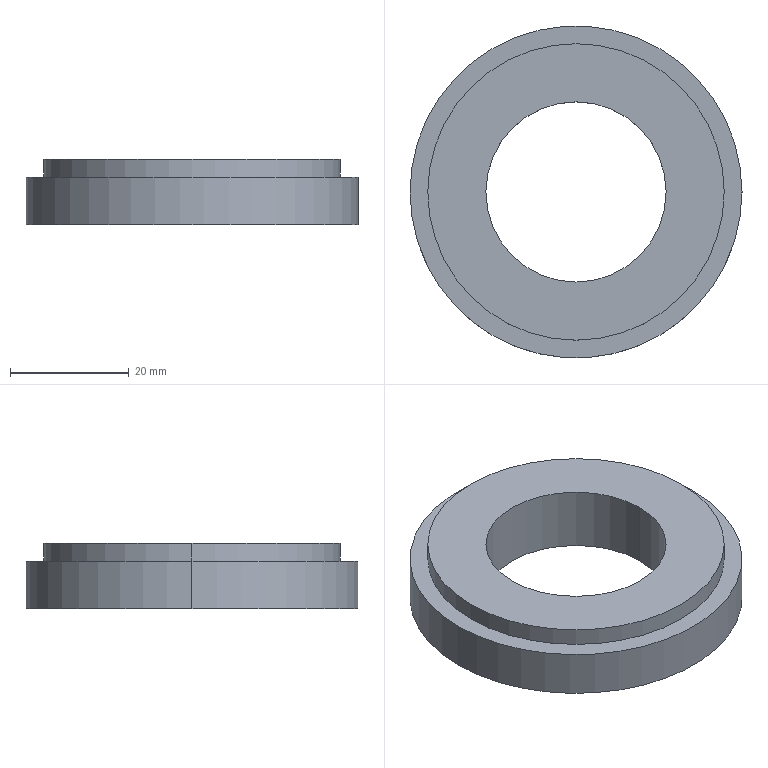Part | SolidWorks | features ICE 2, Extrusion 1 | 1 solid | 9 faces | box 56 x 56 x 11 mm | volume 17612 mm3 | cylinder 6 | plane 3 | commonest cylinder face diameters 30.397 x2 50 x2 56 x2
STEP:
#1=CARTESIAN_POINT('',(15.199,0.,11.));
#2=VERTEX_POINT('',#1);
#3=CARTESIAN_POINT('',(-15.199,0.,11.));
#4=VERTEX_POINT('',#3);
#5=CARTESIAN_POINT('',(0.,0.,11.));
#6=DIRECTION('',(0.,0.,-1.));
#7=DIRECTION('',(-1.,0.,0.));
#8=AXIS2_PLACEMENT_3D('',#5,#6,#7);
#9=CIRCLE('',#8,15.199);
#10=EDGE_CURVE('',#2,#4,#9,.T.);
#11=ORIENTED_EDGE('',*,*,#10,.F.);
#12=CARTESIAN_POINT('',(15.199,0.,0.));
#13=VERTEX_POINT('',#12);
#14=CARTESIAN_POINT('',(15.199,0.,11.));
#15=DIRECTION('',(0.,0.,-1.));
#16=VECTOR('',#15,1000.);
#17=LINE('',#14,#16);
#18=EDGE_CURVE('',#2,#13,#17,.T.);
#19=ORIENTED_EDGE('',*,*,#18,.T.);
#20=CARTESIAN_POINT('',(-15.199,0.,0.));
#21=VERTEX_POINT('',#20);
#22=CARTESIAN_POINT('',(0.,0.,0.));
#23=DIRECTION('',(0.,0.,-1.));
#24=DIRECTION('',(-1.,0.,0.));
#25=AXIS2_PLACEMENT_3D('',#22,#23,#24);
#26=CIRCLE('',#25,15.199);
#27=EDGE_CURVE('',#13,#21,#26,.T.);
#28=ORIENTED_EDGE('',*,*,#27,.T.);
#29=CARTESIAN_POINT('',(-15.199,0.,11.));
#30=DIRECTION('',(0.,0.,-1.));
#31=VECTOR('',#30,1000.);
#32=LINE('',#29,#31);
#33=EDGE_CURVE('',#4,#21,#32,.T.);
#34=ORIENTED_EDGE('',*,*,#33,.F.);
#35=EDGE_LOOP('',(#11,#19,#28,#34));
#36=FACE_OUTER_BOUND('',#35,.T.);
#37=CARTESIAN_POINT('',(0.,0.,11.));
#38=DIRECTION('',(0.,0.,-1.));
#39=DIRECTION('',(-1.,0.,0.));
#40=AXIS2_PLACEMENT_3D('',#37,#38,#39);
#41=CYLINDRICAL_SURFACE('',#40,15.199);
#42=ADVANCED_FACE('',(#36),#41,.F.);
#43=CARTESIAN_POINT('',(25.,0.,11.));
#44=VERTEX_POINT('',#43);
#45=CARTESIAN_POINT('',(-25.,0.,11.));
#46=VERTEX_POINT('',#45);
#47=CARTESIAN_POINT('',(0.,0.,11.));
#48=DIRECTION('',(0.,0.,1.));
#49=DIRECTION('',(1.,0.,0.));
#50=AXIS2_PLACEMENT_3D('',#47,#48,#49);
#51=CIRCLE('',#50,25.);
#52=EDGE_CURVE('',#44,#46,#51,.T.);
#53=ORIENTED_EDGE('',*,*,#52,.F.);
#54=CARTESIAN_POINT('',(25.,0.,8.));
#55=VERTEX_POINT('',#54);
#56=CARTESIAN_POINT('',(25.,0.,11.));
#57=DIRECTION('',(0.,0.,-1.));
#58=VECTOR('',#57,1000.);
#59=LINE('',#56,#58);
#60=EDGE_CURVE('',#44,#55,#59,.T.);
#61=ORIENTED_EDGE('',*,*,#60,.T.);
#62=CARTESIAN_POINT('',(-25.,0.,8.));
#63=VERTEX_POINT('',#62);
#64=CARTESIAN_POINT('',(0.,0.,8.));
#65=DIRECTION('',(0.,0.,1.));
#66=DIRECTION('',(1.,0.,0.));
#67=AXIS2_PLACEMENT_3D('',#64,#65,#66);
#68=CIRCLE('',#67,25.);
#69=EDGE_CURVE('',#55,#63,#68,.T.);
#70=ORIENTED_EDGE('',*,*,#69,.T.);
#71=CARTESIAN_POINT('',(-25.,0.,11.));
#72=DIRECTION('',(0.,0.,-1.));
#73=VECTOR('',#72,1000.);
#74=LINE('',#71,#73);
#75=EDGE_CURVE('',#46,#63,#74,.T.);
#76=ORIENTED_EDGE('',*,*,#75,.F.);
#77=EDGE_LOOP('',(#53,#61,#70,#76));
#78=FACE_OUTER_BOUND('',#77,.T.);
#79=CARTESIAN_POINT('',(0.,0.,11.));
#80=DIRECTION('',(0.,0.,-1.));
#81=DIRECTION('',(-1.,0.,0.));
#82=AXIS2_PLACEMENT_3D('',#79,#80,#81);
#83=CYLINDRICAL_SURFACE('',#82,25.);
#84=ADVANCED_FACE('',(#78),#83,.T.);
#85=CARTESIAN_POINT('',(28.,0.,8.));
#86=VERTEX_POINT('',#85);
#87=CARTESIAN_POINT('',(-28.,0.,8.));
#88=VERTEX_POINT('',#87);
#89=CARTESIAN_POINT('',(0.,0.,8.));
#90=DIRECTION('',(0.,0.,1.));
#91=DIRECTION('',(1.,0.,0.));
#92=AXIS2_PLACEMENT_3D('',#89,#90,#91);
#93=CIRCLE('',#92,28.);
#94=EDGE_CURVE('',#86,#88,#93,.T.);
#95=ORIENTED_EDGE('',*,*,#94,.F.);
#96=CARTESIAN_POINT('',(28.,0.,0.));
#97=VERTEX_POINT('',#96);
#98=CARTESIAN_POINT('',(28.,0.,8.));
#99=DIRECTION('',(0.,0.,-1.));
#100=VECTOR('',#99,1000.);
#101=LINE('',#98,#100);
#102=EDGE_CURVE('',#86,#97,#101,.T.);
#103=ORIENTED_EDGE('',*,*,#102,.T.);
#104=CARTESIAN_POINT('',(-28.,0.,0.));
#105=VERTEX_POINT('',#104);
#106=CARTESIAN_POINT('',(0.,0.,0.));
#107=DIRECTION('',(0.,0.,1.));
#108=DIRECTION('',(1.,0.,0.));
#109=AXIS2_PLACEMENT_3D('',#106,#107,#108);
#110=CIRCLE('',#109,28.);
#111=EDGE_CURVE('',#97,#105,#110,.T.);
#112=ORIENTED_EDGE('',*,*,#111,.T.);
#113=CARTESIAN_POINT('',(-28.,0.,8.));
#114=DIRECTION('',(0.,0.,-1.));
#115=VECTOR('',#114,1000.);
#116=LINE('',#113,#115);
#117=EDGE_CURVE('',#88,#105,#116,.T.);
#118=ORIENTED_EDGE('',*,*,#117,.F.);
#119=EDGE_LOOP('',(#95,#103,#112,#118));
#120=FACE_OUTER_BOUND('',#119,.T.);
#121=CARTESIAN_POINT('',(0.,0.,8.));
#122=DIRECTION('',(0.,0.,-1.));
#123=DIRECTION('',(-1.,0.,0.));
#124=AXIS2_PLACEMENT_3D('',#121,#122,#123);
#125=CYLINDRICAL_SURFACE('',#124,28.);
#126=ADVANCED_FACE('',(#120),#125,.T.);
#127=CARTESIAN_POINT('',(0.,0.,8.));
#128=DIRECTION('',(0.,0.,1.));
#129=DIRECTION('',(1.,0.,0.));
#130=AXIS2_PLACEMENT_3D('',#127,#128,#129);
#131=CIRCLE('',#130,28.);
#132=EDGE_CURVE('',#88,#86,#131,.T.);
#133=ORIENTED_EDGE('',*,*,#132,.T.);
#134=ORIENTED_EDGE('',*,*,#94,.T.);
#135=EDGE_LOOP('',(#133,#134));
#136=FACE_OUTER_BOUND('',#135,.T.);
#137=CARTESIAN_POINT('',(0.,0.,8.));
#138=DIRECTION('',(0.,0.,1.));
#139=DIRECTION('',(1.,0.,0.));
#140=AXIS2_PLACEMENT_3D('',#137,#138,#139);
#141=CIRCLE('',#140,25.);
#142=EDGE_CURVE('',#63,#55,#141,.T.);
#143=ORIENTED_EDGE('',*,*,#142,.F.);
#144=ORIENTED_EDGE('',*,*,#69,.F.);
#145=EDGE_LOOP('',(#143,#144));
#146=FACE_BOUND('',#145,.T.);
#147=CARTESIAN_POINT('',(0.,0.,8.));
#148=DIRECTION('',(0.,0.,1.));
#149=DIRECTION('',(1.,0.,0.));
#150=AXIS2_PLACEMENT_3D('',#147,#148,#149);
#151=PLANE('',#150);
#152=ADVANCED_FACE('',(#136,#146),#151,.T.);
#153=ORIENTED_EDGE('',*,*,#102,.F.);
#154=ORIENTED_EDGE('',*,*,#132,.F.);
#155=ORIENTED_EDGE('',*,*,#117,.T.);
#156=CARTESIAN_POINT('',(0.,0.,0.));
#157=DIRECTION('',(0.,0.,1.));
#158=DIRECTION('',(1.,0.,0.));
#159=AXIS2_PLACEMENT_3D('',#156,#157,#158);
#160=CIRCLE('',#159,28.);
#161=EDGE_CURVE('',#105,#97,#160,.T.);
#162=ORIENTED_EDGE('',*,*,#161,.T.);
#163=EDGE_LOOP('',(#153,#154,#155,#162));
#164=FACE_OUTER_BOUND('',#163,.T.);
#165=CARTESIAN_POINT('',(0.,0.,8.));
#166=DIRECTION('',(0.,0.,-1.));
#167=DIRECTION('',(-1.,0.,0.));
#168=AXIS2_PLACEMENT_3D('',#165,#166,#167);
#169=CYLINDRICAL_SURFACE('',#168,28.);
#170=ADVANCED_FACE('',(#164),#169,.T.);
#171=CARTESIAN_POINT('',(0.,0.,0.));
#172=DIRECTION('',(0.,0.,-1.));
#173=DIRECTION('',(-1.,0.,0.));
#174=AXIS2_PLACEMENT_3D('',#171,#172,#173);
#175=CIRCLE('',#174,15.199);
#176=EDGE_CURVE('',#21,#13,#175,.T.);
#177=ORIENTED_EDGE('',*,*,#176,.F.);
#178=ORIENTED_EDGE('',*,*,#27,.F.);
#179=EDGE_LOOP('',(#177,#178));
#180=FACE_BOUND('',#179,.T.);
#181=ORIENTED_EDGE('',*,*,#161,.F.);
#182=ORIENTED_EDGE('',*,*,#111,.F.);
#183=EDGE_LOOP('',(#181,#182));
#184=FACE_OUTER_BOUND('',#183,.T.);
#185=CARTESIAN_POINT('',(0.,0.,0.));
#186=DIRECTION('',(0.,0.,1.));
#187=DIRECTION('',(1.,0.,0.));
#188=AXIS2_PLACEMENT_3D('',#185,#186,#187);
#189=PLANE('',#188);
#190=ADVANCED_FACE('',(#180,#184),#189,.F.);
#191=ORIENTED_EDGE('',*,*,#60,.F.);
#192=CARTESIAN_POINT('',(0.,0.,11.));
#193=DIRECTION('',(0.,0.,1.));
#194=DIRECTION('',(1.,0.,0.));
#195=AXIS2_PLACEMENT_3D('',#192,#193,#194);
#196=CIRCLE('',#195,25.);
#197=EDGE_CURVE('',#46,#44,#196,.T.);
#198=ORIENTED_EDGE('',*,*,#197,.F.);
#199=ORIENTED_EDGE('',*,*,#75,.T.);
#200=ORIENTED_EDGE('',*,*,#142,.T.);
#201=EDGE_LOOP('',(#191,#198,#199,#200));
#202=FACE_OUTER_BOUND('',#201,.T.);
#203=CARTESIAN_POINT('',(0.,0.,11.));
#204=DIRECTION('',(0.,0.,-1.));
#205=DIRECTION('',(-1.,0.,0.));
#206=AXIS2_PLACEMENT_3D('',#203,#204,#205);
#207=CYLINDRICAL_SURFACE('',#206,25.);
#208=ADVANCED_FACE('',(#202),#207,.T.);
#209=CARTESIAN_POINT('',(0.,0.,11.));
#210=DIRECTION('',(0.,0.,-1.));
#211=DIRECTION('',(-1.,0.,0.));
#212=AXIS2_PLACEMENT_3D('',#209,#210,#211);
#213=CIRCLE('',#212,15.199);
#214=EDGE_CURVE('',#4,#2,#213,.T.);
#215=ORIENTED_EDGE('',*,*,#214,.T.);
#216=ORIENTED_EDGE('',*,*,#10,.T.);
#217=EDGE_LOOP('',(#215,#216));
#218=FACE_BOUND('',#217,.T.);
#219=ORIENTED_EDGE('',*,*,#197,.T.);
#220=ORIENTED_EDGE('',*,*,#52,.T.);
#221=EDGE_LOOP('',(#219,#220));
#222=FACE_OUTER_BOUND('',#221,.T.);
#223=CARTESIAN_POINT('',(0.,0.,11.));
#224=DIRECTION('',(0.,0.,1.));
#225=DIRECTION('',(1.,0.,0.));
#226=AXIS2_PLACEMENT_3D('',#223,#224,#225);
#227=PLANE('',#226);
#228=ADVANCED_FACE('',(#218,#222),#227,.T.);
#229=ORIENTED_EDGE('',*,*,#18,.F.);
#230=ORIENTED_EDGE('',*,*,#214,.F.);
#231=ORIENTED_EDGE('',*,*,#33,.T.);
#232=ORIENTED_EDGE('',*,*,#176,.T.);
#233=EDGE_LOOP('',(#229,#230,#231,#232));
#234=FACE_OUTER_BOUND('',#233,.T.);
#235=CARTESIAN_POINT('',(0.,0.,11.));
#236=DIRECTION('',(0.,0.,-1.));
#237=DIRECTION('',(-1.,0.,0.));
#238=AXIS2_PLACEMENT_3D('',#235,#236,#237);
#239=CYLINDRICAL_SURFACE('',#238,15.199);
#240=ADVANCED_FACE('',(#234),#239,.F.);
#241=CLOSED_SHELL('',(#42,#84,#126,#152,#170,#190,#208,#228,#240));
#242=MANIFOLD_SOLID_BREP('',#241);
#243=CARTESIAN_POINT('',(0.,0.,0.));
#244=DIRECTION('',(0.,0.,1.));
#245=DIRECTION('',(1.,0.,0.));
#246=AXIS2_PLACEMENT_3D('',#243,#244,#245);
#247=(LENGTH_UNIT()NAMED_UNIT(*)SI_UNIT(.MILLI.,.METRE.));
#248=UNCERTAINTY_MEASURE_WITH_UNIT(LENGTH_MEASURE(0.00001),#247,'','');
#249=(NAMED_UNIT(*)PLANE_ANGLE_UNIT()SI_UNIT($,.RADIAN.));
#250=(NAMED_UNIT(*)SI_UNIT($,.STERADIAN.)SOLID_ANGLE_UNIT());
#251=(GEOMETRIC_REPRESENTATION_CONTEXT(3)GLOBAL_UNCERTAINTY_ASSIGNED_CONTEXT((#248))GLOBAL_UNIT_ASSIGNED_CONTEXT((#247,#249,#250))REPRESENTATION_CONTEXT('',''));
#252=ADVANCED_BREP_SHAPE_REPRESENTATION('',(#242,#246),#251);